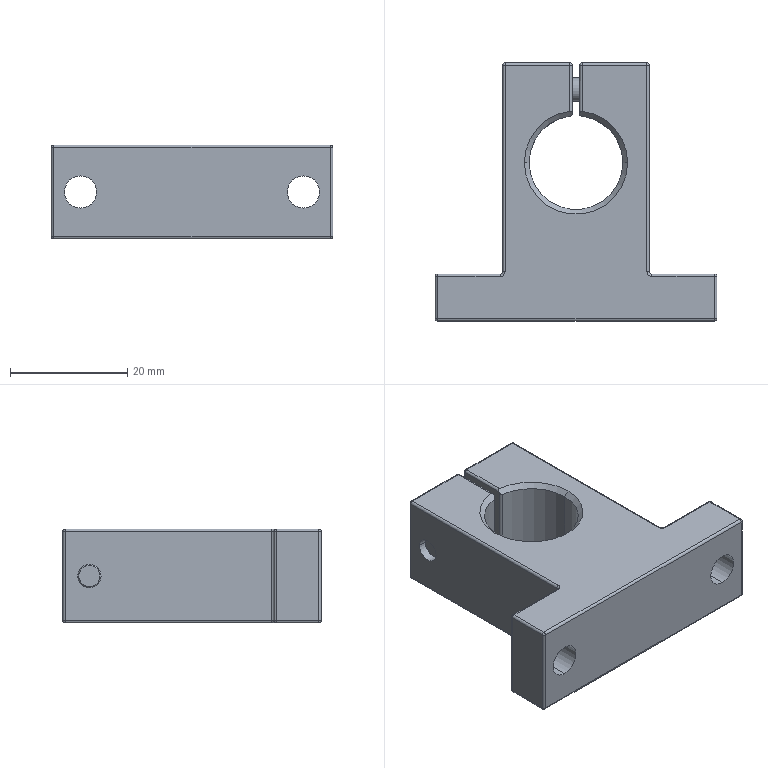Part | NX | features BREP 2 | 2 solids | 110 faces | box 48 x 44 x 16 mm | volume 16689 mm3 | cylinder 51 | plane 25 | sphere 16 | cone 12 | torus 6 | commonest cylinder face diameters 0.8 x34 4 x6 5.5 x4 16 x3 5.2 x2 5.46 x2